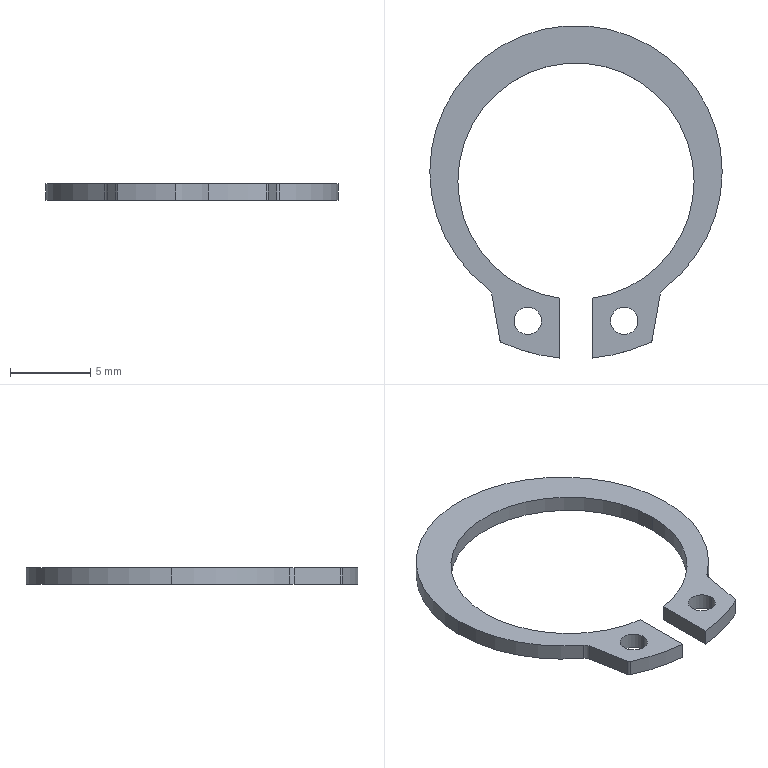Part | SolidWorks | features MoveCopyBody 1, Stock 1 | 1 solid | 22 faces | box 18.2 x 20.685 x 1 mm | volume 104.691 mm3 | cylinder 16 | plane 6 | commonest cylinder face diameters 1.7 x4 14.7 x3 18.2 x3 0.4 x2 1 x2 22.1 x2
STEP:
#1=CARTESIAN_POINT('',(2.15,-8.697,0.));
#2=VERTEX_POINT('',#1);
#3=CARTESIAN_POINT('',(3.85,-8.697,0.));
#4=VERTEX_POINT('',#3);
#5=CARTESIAN_POINT('',(3.,-8.697,0.));
#6=DIRECTION('',(0.,0.,1.));
#7=DIRECTION('',(-1.,0.,0.));
#8=AXIS2_PLACEMENT_3D('',#5,#6,#7);
#9=CIRCLE('',#8,0.85);
#10=EDGE_CURVE('',#2,#4,#9,.T.);
#11=ORIENTED_EDGE('',*,*,#10,.F.);
#12=CARTESIAN_POINT('',(2.15,-8.697,1.));
#13=VERTEX_POINT('',#12);
#14=CARTESIAN_POINT('',(2.15,-8.697,0.));
#15=DIRECTION('',(0.,0.,1.));
#16=VECTOR('',#15,1000.);
#17=LINE('',#14,#16);
#18=EDGE_CURVE('',#2,#13,#17,.T.);
#19=ORIENTED_EDGE('',*,*,#18,.T.);
#20=CARTESIAN_POINT('',(3.85,-8.697,1.));
#21=VERTEX_POINT('',#20);
#22=CARTESIAN_POINT('',(3.,-8.697,1.));
#23=DIRECTION('',(0.,0.,1.));
#24=DIRECTION('',(-1.,0.,0.));
#25=AXIS2_PLACEMENT_3D('',#22,#23,#24);
#26=CIRCLE('',#25,0.85);
#27=EDGE_CURVE('',#13,#21,#26,.T.);
#28=ORIENTED_EDGE('',*,*,#27,.T.);
#29=CARTESIAN_POINT('',(3.85,-8.697,0.));
#30=DIRECTION('',(0.,0.,1.));
#31=VECTOR('',#30,1000.);
#32=LINE('',#29,#31);
#33=EDGE_CURVE('',#4,#21,#32,.T.);
#34=ORIENTED_EDGE('',*,*,#33,.F.);
#35=EDGE_LOOP('',(#11,#19,#28,#34));
#36=FACE_OUTER_BOUND('',#35,.T.);
#37=CARTESIAN_POINT('',(3.,-8.697,0.));
#38=DIRECTION('',(0.,0.,1.));
#39=DIRECTION('',(1.,0.,0.));
#40=AXIS2_PLACEMENT_3D('',#37,#38,#39);
#41=CYLINDRICAL_SURFACE('',#40,0.85);
#42=ADVANCED_FACE('',(#36),#41,.F.);
#43=CARTESIAN_POINT('',(-3.85,-8.697,0.));
#44=VERTEX_POINT('',#43);
#45=CARTESIAN_POINT('',(-2.15,-8.697,0.));
#46=VERTEX_POINT('',#45);
#47=CARTESIAN_POINT('',(-3.,-8.697,0.));
#48=DIRECTION('',(0.,0.,1.));
#49=DIRECTION('',(1.,0.,0.));
#50=AXIS2_PLACEMENT_3D('',#47,#48,#49);
#51=CIRCLE('',#50,0.85);
#52=EDGE_CURVE('',#44,#46,#51,.T.);
#53=ORIENTED_EDGE('',*,*,#52,.F.);
#54=CARTESIAN_POINT('',(-3.85,-8.697,1.));
#55=VERTEX_POINT('',#54);
#56=CARTESIAN_POINT('',(-3.85,-8.697,0.));
#57=DIRECTION('',(0.,0.,1.));
#58=VECTOR('',#57,1000.);
#59=LINE('',#56,#58);
#60=EDGE_CURVE('',#44,#55,#59,.T.);
#61=ORIENTED_EDGE('',*,*,#60,.T.);
#62=CARTESIAN_POINT('',(-2.15,-8.697,1.));
#63=VERTEX_POINT('',#62);
#64=CARTESIAN_POINT('',(-3.,-8.697,1.));
#65=DIRECTION('',(0.,0.,1.));
#66=DIRECTION('',(1.,0.,0.));
#67=AXIS2_PLACEMENT_3D('',#64,#65,#66);
#68=CIRCLE('',#67,0.85);
#69=EDGE_CURVE('',#55,#63,#68,.T.);
#70=ORIENTED_EDGE('',*,*,#69,.T.);
#71=CARTESIAN_POINT('',(-2.15,-8.697,0.));
#72=DIRECTION('',(0.,0.,1.));
#73=VECTOR('',#72,1000.);
#74=LINE('',#71,#73);
#75=EDGE_CURVE('',#46,#63,#74,.T.);
#76=ORIENTED_EDGE('',*,*,#75,.F.);
#77=EDGE_LOOP('',(#53,#61,#70,#76));
#78=FACE_OUTER_BOUND('',#77,.T.);
#79=CARTESIAN_POINT('',(-3.,-8.697,0.));
#80=DIRECTION('',(0.,0.,1.));
#81=DIRECTION('',(1.,0.,0.));
#82=AXIS2_PLACEMENT_3D('',#79,#80,#81);
#83=CYLINDRICAL_SURFACE('',#82,0.85);
#84=ADVANCED_FACE('',(#78),#83,.F.);
#85=CARTESIAN_POINT('',(9.1,0.58,0.));
#86=VERTEX_POINT('',#85);
#87=CARTESIAN_POINT('',(-9.1,0.58,0.));
#88=VERTEX_POINT('',#87);
#89=CARTESIAN_POINT('',(0.,0.58,0.));
#90=DIRECTION('',(0.,0.,1.));
#91=DIRECTION('',(1.,0.,0.));
#92=AXIS2_PLACEMENT_3D('',#89,#90,#91);
#93=CIRCLE('',#92,9.1);
#94=EDGE_CURVE('',#86,#88,#93,.T.);
#95=ORIENTED_EDGE('',*,*,#94,.T.);
#96=CARTESIAN_POINT('',(-9.1,0.58,1.));
#97=VERTEX_POINT('',#96);
#98=CARTESIAN_POINT('',(-9.1,0.58,0.));
#99=DIRECTION('',(0.,0.,1.));
#100=VECTOR('',#99,1000.);
#101=LINE('',#98,#100);
#102=EDGE_CURVE('',#88,#97,#101,.T.);
#103=ORIENTED_EDGE('',*,*,#102,.T.);
#104=CARTESIAN_POINT('',(9.1,0.58,1.));
#105=VERTEX_POINT('',#104);
#106=CARTESIAN_POINT('',(0.,0.58,1.));
#107=DIRECTION('',(0.,0.,1.));
#108=DIRECTION('',(1.,0.,0.));
#109=AXIS2_PLACEMENT_3D('',#106,#107,#108);
#110=CIRCLE('',#109,9.1);
#111=EDGE_CURVE('',#105,#97,#110,.T.);
#112=ORIENTED_EDGE('',*,*,#111,.F.);
#113=CARTESIAN_POINT('',(9.1,0.58,0.));
#114=DIRECTION('',(0.,0.,1.));
#115=VECTOR('',#114,1000.);
#116=LINE('',#113,#115);
#117=EDGE_CURVE('',#86,#105,#116,.T.);
#118=ORIENTED_EDGE('',*,*,#117,.F.);
#119=EDGE_LOOP('',(#95,#103,#112,#118));
#120=FACE_OUTER_BOUND('',#119,.T.);
#121=CARTESIAN_POINT('',(0.,0.58,0.));
#122=DIRECTION('',(0.,0.,1.));
#123=DIRECTION('',(1.,0.,0.));
#124=AXIS2_PLACEMENT_3D('',#121,#122,#123);
#125=CYLINDRICAL_SURFACE('',#124,9.1);
#126=ADVANCED_FACE('',(#120),#125,.T.);
#127=CARTESIAN_POINT('',(5.437,-6.717,0.));
#128=VERTEX_POINT('',#127);
#129=CARTESIAN_POINT('',(0.,0.58,0.));
#130=DIRECTION('',(0.,0.,1.));
#131=DIRECTION('',(1.,0.,0.));
#132=AXIS2_PLACEMENT_3D('',#129,#130,#131);
#133=CIRCLE('',#132,9.1);
#134=EDGE_CURVE('',#128,#86,#133,.T.);
#135=ORIENTED_EDGE('',*,*,#134,.T.);
#136=ORIENTED_EDGE('',*,*,#117,.T.);
#137=CARTESIAN_POINT('',(5.437,-6.717,1.));
#138=VERTEX_POINT('',#137);
#139=CARTESIAN_POINT('',(0.,0.58,1.));
#140=DIRECTION('',(0.,0.,1.));
#141=DIRECTION('',(1.,0.,0.));
#142=AXIS2_PLACEMENT_3D('',#139,#140,#141);
#143=CIRCLE('',#142,9.1);
#144=EDGE_CURVE('',#138,#105,#143,.T.);
#145=ORIENTED_EDGE('',*,*,#144,.F.);
#146=CARTESIAN_POINT('',(5.437,-6.717,0.));
#147=DIRECTION('',(0.,0.,-1.));
#148=VECTOR('',#147,1000.);
#149=LINE('',#146,#148);
#150=EDGE_CURVE('',#138,#128,#149,.T.);
#151=ORIENTED_EDGE('',*,*,#150,.T.);
#152=EDGE_LOOP('',(#135,#136,#145,#151));
#153=FACE_OUTER_BOUND('',#152,.T.);
#154=CARTESIAN_POINT('',(0.,0.58,0.));
#155=DIRECTION('',(0.,0.,1.));
#156=DIRECTION('',(1.,0.,0.));
#157=AXIS2_PLACEMENT_3D('',#154,#155,#156);
#158=CYLINDRICAL_SURFACE('',#157,9.1);
#159=ADVANCED_FACE('',(#153),#158,.T.);
#160=CARTESIAN_POINT('',(-1.,-7.282,0.));
#161=VERTEX_POINT('',#160);
#162=CARTESIAN_POINT('',(-7.35,0.,0.));
#163=VERTEX_POINT('',#162);
#164=CARTESIAN_POINT('',(0.,0.,0.));
#165=DIRECTION('',(0.,0.,-1.));
#166=DIRECTION('',(1.,0.,0.));
#167=AXIS2_PLACEMENT_3D('',#164,#165,#166);
#168=CIRCLE('',#167,7.35);
#169=EDGE_CURVE('',#161,#163,#168,.T.);
#170=ORIENTED_EDGE('',*,*,#169,.T.);
#171=CARTESIAN_POINT('',(-7.35,0.,1.));
#172=VERTEX_POINT('',#171);
#173=CARTESIAN_POINT('',(-7.35,0.,0.));
#174=DIRECTION('',(0.,0.,1.));
#175=VECTOR('',#174,1000.);
#176=LINE('',#173,#175);
#177=EDGE_CURVE('',#163,#172,#176,.T.);
#178=ORIENTED_EDGE('',*,*,#177,.T.);
#179=CARTESIAN_POINT('',(-1.,-7.282,1.));
#180=VERTEX_POINT('',#179);
#181=CARTESIAN_POINT('',(0.,0.,1.));
#182=DIRECTION('',(0.,0.,-1.));
#183=DIRECTION('',(1.,0.,0.));
#184=AXIS2_PLACEMENT_3D('',#181,#182,#183);
#185=CIRCLE('',#184,7.35);
#186=EDGE_CURVE('',#180,#172,#185,.T.);
#187=ORIENTED_EDGE('',*,*,#186,.F.);
#188=CARTESIAN_POINT('',(-1.,-7.282,0.));
#189=DIRECTION('',(0.,0.,1.));
#190=VECTOR('',#189,1000.);
#191=LINE('',#188,#190);
#192=EDGE_CURVE('',#161,#180,#191,.T.);
#193=ORIENTED_EDGE('',*,*,#192,.F.);
#194=EDGE_LOOP('',(#170,#178,#187,#193));
#195=FACE_OUTER_BOUND('',#194,.T.);
#196=CARTESIAN_POINT('',(0.,0.,0.));
#197=DIRECTION('',(0.,0.,1.));
#198=DIRECTION('',(1.,0.,0.));
#199=AXIS2_PLACEMENT_3D('',#196,#197,#198);
#200=CYLINDRICAL_SURFACE('',#199,7.35);
#201=ADVANCED_FACE('',(#195),#200,.F.);
#202=ORIENTED_EDGE('',*,*,#177,.F.);
#203=CARTESIAN_POINT('',(7.35,0.,0.));
#204=VERTEX_POINT('',#203);
#205=CARTESIAN_POINT('',(0.,0.,0.));
#206=DIRECTION('',(0.,0.,-1.));
#207=DIRECTION('',(1.,0.,0.));
#208=AXIS2_PLACEMENT_3D('',#205,#206,#207);
#209=CIRCLE('',#208,7.35);
#210=EDGE_CURVE('',#163,#204,#209,.T.);
#211=ORIENTED_EDGE('',*,*,#210,.T.);
#212=CARTESIAN_POINT('',(7.35,0.,1.));
#213=VERTEX_POINT('',#212);
#214=CARTESIAN_POINT('',(7.35,0.,0.));
#215=DIRECTION('',(0.,0.,1.));
#216=VECTOR('',#215,1000.);
#217=LINE('',#214,#216);
#218=EDGE_CURVE('',#204,#213,#217,.T.);
#219=ORIENTED_EDGE('',*,*,#218,.T.);
#220=CARTESIAN_POINT('',(0.,0.,1.));
#221=DIRECTION('',(0.,0.,-1.));
#222=DIRECTION('',(1.,0.,0.));
#223=AXIS2_PLACEMENT_3D('',#220,#221,#222);
#224=CIRCLE('',#223,7.35);
#225=EDGE_CURVE('',#172,#213,#224,.T.);
#226=ORIENTED_EDGE('',*,*,#225,.F.);
#227=EDGE_LOOP('',(#202,#211,#219,#226));
#228=FACE_OUTER_BOUND('',#227,.T.);
#229=CARTESIAN_POINT('',(0.,0.,0.));
#230=DIRECTION('',(0.,0.,1.));
#231=DIRECTION('',(1.,0.,0.));
#232=AXIS2_PLACEMENT_3D('',#229,#230,#231);
#233=CYLINDRICAL_SURFACE('',#232,7.35);
#234=ADVANCED_FACE('',(#228),#233,.F.);
#235=CARTESIAN_POINT('',(1.,-11.005,0.));
#236=VERTEX_POINT('',#235);
#237=CARTESIAN_POINT('',(4.626,-10.035,0.));
#238=VERTEX_POINT('',#237);
#239=CARTESIAN_POINT('',(0.,0.,0.));
#240=DIRECTION('',(0.,0.,1.));
#241=DIRECTION('',(-1.,0.,0.));
#242=AXIS2_PLACEMENT_3D('',#239,#240,#241);
#243=CIRCLE('',#242,11.05);
#244=EDGE_CURVE('',#236,#238,#243,.T.);
#245=ORIENTED_EDGE('',*,*,#244,.T.);
#246=CARTESIAN_POINT('',(4.626,-10.035,1.));
#247=VERTEX_POINT('',#246);
#248=CARTESIAN_POINT('',(4.626,-10.035,0.));
#249=DIRECTION('',(0.,0.,1.));
#250=VECTOR('',#249,1000.);
#251=LINE('',#248,#250);
#252=EDGE_CURVE('',#238,#247,#251,.T.);
#253=ORIENTED_EDGE('',*,*,#252,.T.);
#254=CARTESIAN_POINT('',(1.,-11.005,1.));
#255=VERTEX_POINT('',#254);
#256=CARTESIAN_POINT('',(0.,0.,1.));
#257=DIRECTION('',(0.,0.,1.));
#258=DIRECTION('',(-1.,0.,0.));
#259=AXIS2_PLACEMENT_3D('',#256,#257,#258);
#260=CIRCLE('',#259,11.05);
#261=EDGE_CURVE('',#255,#247,#260,.T.);
#262=ORIENTED_EDGE('',*,*,#261,.F.);
#263=CARTESIAN_POINT('',(1.,-11.005,0.));
#264=DIRECTION('',(0.,0.,1.));
#265=VECTOR('',#264,1000.);
#266=LINE('',#263,#265);
#267=EDGE_CURVE('',#236,#255,#266,.T.);
#268=ORIENTED_EDGE('',*,*,#267,.F.);
#269=EDGE_LOOP('',(#245,#253,#262,#268));
#270=FACE_OUTER_BOUND('',#269,.T.);
#271=CARTESIAN_POINT('',(0.,0.,0.));
#272=DIRECTION('',(0.,0.,1.));
#273=DIRECTION('',(1.,0.,0.));
#274=AXIS2_PLACEMENT_3D('',#271,#272,#273);
#275=CYLINDRICAL_SURFACE('',#274,11.05);
#276=ADVANCED_FACE('',(#270),#275,.T.);
#277=CARTESIAN_POINT('',(1.,-7.282,1.));
#278=VERTEX_POINT('',#277);
#279=CARTESIAN_POINT('',(1.,-7.282,1.));
#280=DIRECTION('',(0.,-1.,0.));
#281=VECTOR('',#280,1000.);
#282=LINE('',#279,#281);
#283=EDGE_CURVE('',#278,#255,#282,.T.);
#284=ORIENTED_EDGE('',*,*,#283,.F.);
#285=CARTESIAN_POINT('',(1.,-7.282,0.));
#286=VERTEX_POINT('',#285);
#287=CARTESIAN_POINT('',(1.,-7.282,0.));
#288=DIRECTION('',(0.,0.,1.));
#289=VECTOR('',#288,1000.);
#290=LINE('',#287,#289);
#291=EDGE_CURVE('',#286,#278,#290,.T.);
#292=ORIENTED_EDGE('',*,*,#291,.F.);
#293=CARTESIAN_POINT('',(1.,-7.282,0.));
#294=DIRECTION('',(0.,-1.,0.));
#295=VECTOR('',#294,1000.);
#296=LINE('',#293,#295);
#297=EDGE_CURVE('',#286,#236,#296,.T.);
#298=ORIENTED_EDGE('',*,*,#297,.T.);
#299=ORIENTED_EDGE('',*,*,#267,.T.);
#300=EDGE_LOOP('',(#284,#292,#298,#299));
#301=FACE_OUTER_BOUND('',#300,.T.);
#302=CARTESIAN_POINT('',(1.,-7.282,0.));
#303=DIRECTION('',(-1.,0.,0.));
#304=DIRECTION('',(0.,0.,1.));
#305=AXIS2_PLACEMENT_3D('',#302,#303,#304);
#306=PLANE('',#305);
#307=ADVANCED_FACE('',(#301),#306,.T.);
#308=ORIENTED_EDGE('',*,*,#218,.F.);
#309=CARTESIAN_POINT('',(0.,0.,0.));
#310=DIRECTION('',(0.,0.,-1.));
#311=DIRECTION('',(1.,0.,0.));
#312=AXIS2_PLACEMENT_3D('',#309,#310,#311);
#313=CIRCLE('',#312,7.35);
#314=EDGE_CURVE('',#204,#286,#313,.T.);
#315=ORIENTED_EDGE('',*,*,#314,.T.);
#316=ORIENTED_EDGE('',*,*,#291,.T.);
#317=CARTESIAN_POINT('',(0.,0.,1.));
#318=DIRECTION('',(0.,0.,-1.));
#319=DIRECTION('',(1.,0.,0.));
#320=AXIS2_PLACEMENT_3D('',#317,#318,#319);
#321=CIRCLE('',#320,7.35);
#322=EDGE_CURVE('',#213,#278,#321,.T.);
#323=ORIENTED_EDGE('',*,*,#322,.F.);
#324=EDGE_LOOP('',(#308,#315,#316,#323));
#325=FACE_OUTER_BOUND('',#324,.T.);
#326=CARTESIAN_POINT('',(0.,0.,0.));
#327=DIRECTION('',(0.,0.,1.));
#328=DIRECTION('',(1.,0.,0.));
#329=AXIS2_PLACEMENT_3D('',#326,#327,#328);
#330=CYLINDRICAL_SURFACE('',#329,7.35);
#331=ADVANCED_FACE('',(#325),#330,.F.);
#332=CARTESIAN_POINT('',(-1.,-11.005,1.));
#333=VERTEX_POINT('',#332);
#334=CARTESIAN_POINT('',(-1.,-7.282,1.));
#335=DIRECTION('',(0.,1.,0.));
#336=VECTOR('',#335,1000.);
#337=LINE('',#334,#336);
#338=EDGE_CURVE('',#333,#180,#337,.T.);
#339=ORIENTED_EDGE('',*,*,#338,.F.);
#340=CARTESIAN_POINT('',(-1.,-11.005,0.));
#341=VERTEX_POINT('',#340);
#342=CARTESIAN_POINT('',(-1.,-11.005,0.));
#343=DIRECTION('',(0.,0.,1.));
#344=VECTOR('',#343,1000.);
#345=LINE('',#342,#344);
#346=EDGE_CURVE('',#341,#333,#345,.T.);
#347=ORIENTED_EDGE('',*,*,#346,.F.);
#348=CARTESIAN_POINT('',(-1.,-7.282,0.));
#349=DIRECTION('',(0.,1.,0.));
#350=VECTOR('',#349,1000.);
#351=LINE('',#348,#350);
#352=EDGE_CURVE('',#341,#161,#351,.T.);
#353=ORIENTED_EDGE('',*,*,#352,.T.);
#354=ORIENTED_EDGE('',*,*,#192,.T.);
#355=EDGE_LOOP('',(#339,#347,#353,#354));
#356=FACE_OUTER_BOUND('',#355,.T.);
#357=CARTESIAN_POINT('',(-1.,-7.282,0.));
#358=DIRECTION('',(1.,0.,0.));
#359=DIRECTION('',(0.,0.,-1.));
#360=AXIS2_PLACEMENT_3D('',#357,#358,#359);
#361=PLANE('',#360);
#362=ADVANCED_FACE('',(#356),#361,.T.);
#363=CARTESIAN_POINT('',(-4.626,-10.035,1.));
#364=VERTEX_POINT('',#363);
#365=CARTESIAN_POINT('',(0.,0.,1.));
#366=DIRECTION('',(0.,0.,1.));
#367=DIRECTION('',(1.,0.,0.));
#368=AXIS2_PLACEMENT_3D('',#365,#366,#367);
#369=CIRCLE('',#368,11.05);
#370=EDGE_CURVE('',#364,#333,#369,.T.);
#371=ORIENTED_EDGE('',*,*,#370,.F.);
#372=CARTESIAN_POINT('',(-4.626,-10.035,0.));
#373=VERTEX_POINT('',#372);
#374=CARTESIAN_POINT('',(-4.626,-10.035,0.));
#375=DIRECTION('',(0.,0.,-1.));
#376=VECTOR('',#375,1000.);
#377=LINE('',#374,#376);
#378=EDGE_CURVE('',#364,#373,#377,.T.);
#379=ORIENTED_EDGE('',*,*,#378,.T.);
#380=CARTESIAN_POINT('',(0.,0.,0.));
#381=DIRECTION('',(0.,0.,1.));
#382=DIRECTION('',(1.,0.,0.));
#383=AXIS2_PLACEMENT_3D('',#380,#381,#382);
#384=CIRCLE('',#383,11.05);
#385=EDGE_CURVE('',#373,#341,#384,.T.);
#386=ORIENTED_EDGE('',*,*,#385,.T.);
#387=ORIENTED_EDGE('',*,*,#346,.T.);
#388=EDGE_LOOP('',(#371,#379,#386,#387));
#389=FACE_OUTER_BOUND('',#388,.T.);
#390=CARTESIAN_POINT('',(0.,0.,0.));
#391=DIRECTION('',(0.,0.,1.));
#392=DIRECTION('',(1.,0.,0.));
#393=AXIS2_PLACEMENT_3D('',#390,#391,#392);
#394=CYLINDRICAL_SURFACE('',#393,11.05);
#395=ADVANCED_FACE('',(#389),#394,.T.);
#396=CARTESIAN_POINT('',(-5.243,-7.031,1.));
#397=VERTEX_POINT('',#396);
#398=CARTESIAN_POINT('',(-4.74,-9.888,1.));
#399=VERTEX_POINT('',#398);
#400=CARTESIAN_POINT('',(-5.278,-6.833,1.));
#401=DIRECTION('',(0.1736,-0.9848,0.));
#402=VECTOR('',#401,1000.);
#403=LINE('',#400,#402);
#404=EDGE_CURVE('',#397,#399,#403,.T.);
#405=ORIENTED_EDGE('',*,*,#404,.F.);
#406=CARTESIAN_POINT('',(-5.243,-7.031,0.));
#407=VERTEX_POINT('',#406);
#408=CARTESIAN_POINT('',(-5.243,-7.031,0.));
#409=DIRECTION('',(0.,0.,-1.));
#410=VECTOR('',#409,1000.);
#411=LINE('',#408,#410);
#412=EDGE_CURVE('',#397,#407,#411,.T.);
#413=ORIENTED_EDGE('',*,*,#412,.T.);
#414=CARTESIAN_POINT('',(-4.74,-9.888,0.));
#415=VERTEX_POINT('',#414);
#416=CARTESIAN_POINT('',(-5.278,-6.833,0.));
#417=DIRECTION('',(0.1736,-0.9848,0.));
#418=VECTOR('',#417,1000.);
#419=LINE('',#416,#418);
#420=EDGE_CURVE('',#407,#415,#419,.T.);
#421=ORIENTED_EDGE('',*,*,#420,.T.);
#422=CARTESIAN_POINT('',(-4.74,-9.888,0.));
#423=DIRECTION('',(0.,0.,1.));
#424=VECTOR('',#423,1000.);
#425=LINE('',#422,#424);
#426=EDGE_CURVE('',#415,#399,#425,.T.);
#427=ORIENTED_EDGE('',*,*,#426,.T.);
#428=EDGE_LOOP('',(#405,#413,#421,#427));
#429=FACE_OUTER_BOUND('',#428,.T.);
#430=CARTESIAN_POINT('',(-5.278,-6.833,0.));
#431=DIRECTION('',(-0.9848,-0.1736,0.));
#432=DIRECTION('',(0.1736,-0.9848,0.));
#433=AXIS2_PLACEMENT_3D('',#430,#431,#432);
#434=PLANE('',#433);
#435=ADVANCED_FACE('',(#429),#434,.T.);
#436=ORIENTED_EDGE('',*,*,#102,.F.);
#437=CARTESIAN_POINT('',(-5.437,-6.717,0.));
#438=VERTEX_POINT('',#437);
#439=CARTESIAN_POINT('',(0.,0.58,0.));
#440=DIRECTION('',(0.,0.,1.));
#441=DIRECTION('',(1.,0.,0.));
#442=AXIS2_PLACEMENT_3D('',#439,#440,#441);
#443=CIRCLE('',#442,9.1);
#444=EDGE_CURVE('',#88,#438,#443,.T.);
#445=ORIENTED_EDGE('',*,*,#444,.T.);
#446=CARTESIAN_POINT('',(-5.437,-6.717,1.));
#447=VERTEX_POINT('',#446);
#448=CARTESIAN_POINT('',(-5.437,-6.717,0.));
#449=DIRECTION('',(0.,0.,1.));
#450=VECTOR('',#449,1000.);
#451=LINE('',#448,#450);
#452=EDGE_CURVE('',#438,#447,#451,.T.);
#453=ORIENTED_EDGE('',*,*,#452,.T.);
#454=CARTESIAN_POINT('',(0.,0.58,1.));
#455=DIRECTION('',(0.,0.,1.));
#456=DIRECTION('',(1.,0.,0.));
#457=AXIS2_PLACEMENT_3D('',#454,#455,#456);
#458=CIRCLE('',#457,9.1);
#459=EDGE_CURVE('',#97,#447,#458,.T.);
#460=ORIENTED_EDGE('',*,*,#459,.F.);
#461=EDGE_LOOP('',(#436,#445,#453,#460));
#462=FACE_OUTER_BOUND('',#461,.T.);
#463=CARTESIAN_POINT('',(0.,0.58,0.));
#464=DIRECTION('',(0.,0.,1.));
#465=DIRECTION('',(1.,0.,0.));
#466=AXIS2_PLACEMENT_3D('',#463,#464,#465);
#467=CYLINDRICAL_SURFACE('',#466,9.1);
#468=ADVANCED_FACE('',(#462),#467,.T.);
#469=CARTESIAN_POINT('',(4.74,-9.888,0.));
#470=VERTEX_POINT('',#469);
#471=CARTESIAN_POINT('',(5.243,-7.031,0.));
#472=VERTEX_POINT('',#471);
#473=CARTESIAN_POINT('',(5.278,-6.833,0.));
#474=DIRECTION('',(0.1736,0.9848,0.));
#475=VECTOR('',#474,1000.);
#476=LINE('',#473,#475);
#477=EDGE_CURVE('',#470,#472,#476,.T.);
#478=ORIENTED_EDGE('',*,*,#477,.T.);
#479=CARTESIAN_POINT('',(5.243,-7.031,1.));
#480=VERTEX_POINT('',#479);
#481=CARTESIAN_POINT('',(5.243,-7.031,1.));
#482=DIRECTION('',(0.,0.,1.));
#483=VECTOR('',#482,1000.);
#484=LINE('',#481,#483);
#485=EDGE_CURVE('',#472,#480,#484,.T.);
#486=ORIENTED_EDGE('',*,*,#485,.T.);
#487=CARTESIAN_POINT('',(4.74,-9.888,1.));
#488=VERTEX_POINT('',#487);
#489=CARTESIAN_POINT('',(5.278,-6.833,1.));
#490=DIRECTION('',(0.1736,0.9848,0.));
#491=VECTOR('',#490,1000.);
#492=LINE('',#489,#491);
#493=EDGE_CURVE('',#488,#480,#492,.T.);
#494=ORIENTED_EDGE('',*,*,#493,.F.);
#495=CARTESIAN_POINT('',(4.74,-9.888,0.));
#496=DIRECTION('',(0.,0.,-1.));
#497=VECTOR('',#496,1000.);
#498=LINE('',#495,#497);
#499=EDGE_CURVE('',#488,#470,#498,.T.);
#500=ORIENTED_EDGE('',*,*,#499,.T.);
#501=EDGE_LOOP('',(#478,#486,#494,#500));
#502=FACE_OUTER_BOUND('',#501,.T.);
#503=CARTESIAN_POINT('',(5.278,-6.833,0.));
#504=DIRECTION('',(0.9848,-0.1736,0.));
#505=DIRECTION('',(0.1736,0.9848,0.));
#506=AXIS2_PLACEMENT_3D('',#503,#504,#505);
#507=PLANE('',#506);
#508=ADVANCED_FACE('',(#502),#507,.T.);
#509=CARTESIAN_POINT('',(3.,-8.697,0.));
#510=DIRECTION('',(0.,0.,1.));
#511=DIRECTION('',(-1.,0.,0.));
#512=AXIS2_PLACEMENT_3D('',#509,#510,#511);
#513=CIRCLE('',#512,0.85);
#514=EDGE_CURVE('',#4,#2,#513,.T.);
#515=ORIENTED_EDGE('',*,*,#514,.T.);
#516=ORIENTED_EDGE('',*,*,#10,.T.);
#517=EDGE_LOOP('',(#515,#516));
#518=FACE_BOUND('',#517,.T.);
#519=CARTESIAN_POINT('',(-3.,-8.697,0.));
#520=DIRECTION('',(0.,0.,1.));
#521=DIRECTION('',(1.,0.,0.));
#522=AXIS2_PLACEMENT_3D('',#519,#520,#521);
#523=CIRCLE('',#522,0.85);
#524=EDGE_CURVE('',#46,#44,#523,.T.);
#525=ORIENTED_EDGE('',*,*,#524,.T.);
#526=ORIENTED_EDGE('',*,*,#52,.T.);
#527=EDGE_LOOP('',(#525,#526));
#528=FACE_BOUND('',#527,.T.);
#529=ORIENTED_EDGE('',*,*,#385,.F.);
#530=CARTESIAN_POINT('',(-4.543,-9.853,0.));
#531=DIRECTION('',(0.,0.,-1.));
#532=DIRECTION('',(-1.,0.,0.));
#533=AXIS2_PLACEMENT_3D('',#530,#531,#532);
#534=CIRCLE('',#533,0.2);
#535=EDGE_CURVE('',#373,#415,#534,.T.);
#536=ORIENTED_EDGE('',*,*,#535,.T.);
#537=ORIENTED_EDGE('',*,*,#420,.F.);
#538=CARTESIAN_POINT('',(-5.736,-7.118,0.));
#539=DIRECTION('',(0.,0.,1.));
#540=DIRECTION('',(-1.,0.,0.));
#541=AXIS2_PLACEMENT_3D('',#538,#539,#540);
#542=CIRCLE('',#541,0.5);
#543=EDGE_CURVE('',#407,#438,#542,.T.);
#544=ORIENTED_EDGE('',*,*,#543,.T.);
#545=ORIENTED_EDGE('',*,*,#444,.F.);
#546=ORIENTED_EDGE('',*,*,#94,.F.);
#547=ORIENTED_EDGE('',*,*,#134,.F.);
#548=CARTESIAN_POINT('',(5.736,-7.118,0.));
#549=DIRECTION('',(0.,0.,1.));
#550=DIRECTION('',(-1.,0.,0.));
#551=AXIS2_PLACEMENT_3D('',#548,#549,#550);
#552=CIRCLE('',#551,0.5);
#553=EDGE_CURVE('',#128,#472,#552,.T.);
#554=ORIENTED_EDGE('',*,*,#553,.T.);
#555=ORIENTED_EDGE('',*,*,#477,.F.);
#556=CARTESIAN_POINT('',(4.543,-9.853,0.));
#557=DIRECTION('',(0.,0.,-1.));
#558=DIRECTION('',(-1.,0.,0.));
#559=AXIS2_PLACEMENT_3D('',#556,#557,#558);
#560=CIRCLE('',#559,0.2);
#561=EDGE_CURVE('',#470,#238,#560,.T.);
#562=ORIENTED_EDGE('',*,*,#561,.T.);
#563=ORIENTED_EDGE('',*,*,#244,.F.);
#564=ORIENTED_EDGE('',*,*,#297,.F.);
#565=ORIENTED_EDGE('',*,*,#314,.F.);
#566=ORIENTED_EDGE('',*,*,#210,.F.);
#567=ORIENTED_EDGE('',*,*,#169,.F.);
#568=ORIENTED_EDGE('',*,*,#352,.F.);
#569=EDGE_LOOP('',(#529,#536,#537,#544,#545,#546,#547,#554,#555,#562,#563,#564,#565,#566,#567,#568));
#570=FACE_OUTER_BOUND('',#569,.T.);
#571=CARTESIAN_POINT('',(0.,0.,0.));
#572=DIRECTION('',(0.,0.,-1.));
#573=DIRECTION('',(-1.,0.,0.));
#574=AXIS2_PLACEMENT_3D('',#571,#572,#573);
#575=PLANE('',#574);
#576=ADVANCED_FACE('',(#518,#528,#570),#575,.T.);
#577=CARTESIAN_POINT('',(3.,-8.697,1.));
#578=DIRECTION('',(0.,0.,1.));
#579=DIRECTION('',(-1.,0.,0.));
#580=AXIS2_PLACEMENT_3D('',#577,#578,#579);
#581=CIRCLE('',#580,0.85);
#582=EDGE_CURVE('',#21,#13,#581,.T.);
#583=ORIENTED_EDGE('',*,*,#582,.F.);
#584=ORIENTED_EDGE('',*,*,#27,.F.);
#585=EDGE_LOOP('',(#583,#584));
#586=FACE_BOUND('',#585,.T.);
#587=CARTESIAN_POINT('',(-3.,-8.697,1.));
#588=DIRECTION('',(0.,0.,1.));
#589=DIRECTION('',(1.,0.,0.));
#590=AXIS2_PLACEMENT_3D('',#587,#588,#589);
#591=CIRCLE('',#590,0.85);
#592=EDGE_CURVE('',#63,#55,#591,.T.);
#593=ORIENTED_EDGE('',*,*,#592,.F.);
#594=ORIENTED_EDGE('',*,*,#69,.F.);
#595=EDGE_LOOP('',(#593,#594));
#596=FACE_BOUND('',#595,.T.);
#597=ORIENTED_EDGE('',*,*,#144,.T.);
#598=ORIENTED_EDGE('',*,*,#111,.T.);
#599=ORIENTED_EDGE('',*,*,#459,.T.);
#600=CARTESIAN_POINT('',(-5.736,-7.118,1.));
#601=DIRECTION('',(0.,0.,-1.));
#602=DIRECTION('',(-1.,0.,0.));
#603=AXIS2_PLACEMENT_3D('',#600,#601,#602);
#604=CIRCLE('',#603,0.5);
#605=EDGE_CURVE('',#447,#397,#604,.T.);
#606=ORIENTED_EDGE('',*,*,#605,.T.);
#607=ORIENTED_EDGE('',*,*,#404,.T.);
#608=CARTESIAN_POINT('',(-4.543,-9.853,1.));
#609=DIRECTION('',(0.,0.,1.));
#610=DIRECTION('',(-1.,0.,0.));
#611=AXIS2_PLACEMENT_3D('',#608,#609,#610);
#612=CIRCLE('',#611,0.2);
#613=EDGE_CURVE('',#399,#364,#612,.T.);
#614=ORIENTED_EDGE('',*,*,#613,.T.);
#615=ORIENTED_EDGE('',*,*,#370,.T.);
#616=ORIENTED_EDGE('',*,*,#338,.T.);
#617=ORIENTED_EDGE('',*,*,#186,.T.);
#618=ORIENTED_EDGE('',*,*,#225,.T.);
#619=ORIENTED_EDGE('',*,*,#322,.T.);
#620=ORIENTED_EDGE('',*,*,#283,.T.);
#621=ORIENTED_EDGE('',*,*,#261,.T.);
#622=CARTESIAN_POINT('',(4.543,-9.853,1.));
#623=DIRECTION('',(0.,0.,1.));
#624=DIRECTION('',(-1.,0.,0.));
#625=AXIS2_PLACEMENT_3D('',#622,#623,#624);
#626=CIRCLE('',#625,0.2);
#627=EDGE_CURVE('',#247,#488,#626,.T.);
#628=ORIENTED_EDGE('',*,*,#627,.T.);
#629=ORIENTED_EDGE('',*,*,#493,.T.);
#630=CARTESIAN_POINT('',(5.736,-7.118,1.));
#631=DIRECTION('',(0.,0.,-1.));
#632=DIRECTION('',(-1.,0.,0.));
#633=AXIS2_PLACEMENT_3D('',#630,#631,#632);
#634=CIRCLE('',#633,0.5);
#635=EDGE_CURVE('',#480,#138,#634,.T.);
#636=ORIENTED_EDGE('',*,*,#635,.T.);
#637=EDGE_LOOP('',(#597,#598,#599,#606,#607,#614,#615,#616,#617,#618,#619,#620,#621,#628,#629,#636));
#638=FACE_OUTER_BOUND('',#637,.T.);
#639=CARTESIAN_POINT('',(0.,0.,1.));
#640=DIRECTION('',(0.,0.,-1.));
#641=DIRECTION('',(-1.,0.,0.));
#642=AXIS2_PLACEMENT_3D('',#639,#640,#641);
#643=PLANE('',#642);
#644=ADVANCED_FACE('',(#586,#596,#638),#643,.F.);
#645=ORIENTED_EDGE('',*,*,#60,.F.);
#646=ORIENTED_EDGE('',*,*,#524,.F.);
#647=ORIENTED_EDGE('',*,*,#75,.T.);
#648=ORIENTED_EDGE('',*,*,#592,.T.);
#649=EDGE_LOOP('',(#645,#646,#647,#648));
#650=FACE_OUTER_BOUND('',#649,.T.);
#651=CARTESIAN_POINT('',(-3.,-8.697,0.));
#652=DIRECTION('',(0.,0.,1.));
#653=DIRECTION('',(1.,0.,0.));
#654=AXIS2_PLACEMENT_3D('',#651,#652,#653);
#655=CYLINDRICAL_SURFACE('',#654,0.85);
#656=ADVANCED_FACE('',(#650),#655,.F.);
#657=ORIENTED_EDGE('',*,*,#18,.F.);
#658=ORIENTED_EDGE('',*,*,#514,.F.);
#659=ORIENTED_EDGE('',*,*,#33,.T.);
#660=ORIENTED_EDGE('',*,*,#582,.T.);
#661=EDGE_LOOP('',(#657,#658,#659,#660));
#662=FACE_OUTER_BOUND('',#661,.T.);
#663=CARTESIAN_POINT('',(3.,-8.697,0.));
#664=DIRECTION('',(0.,0.,1.));
#665=DIRECTION('',(1.,0.,0.));
#666=AXIS2_PLACEMENT_3D('',#663,#664,#665);
#667=CYLINDRICAL_SURFACE('',#666,0.85);
#668=ADVANCED_FACE('',(#662),#667,.F.);
#669=ORIENTED_EDGE('',*,*,#535,.F.);
#670=ORIENTED_EDGE('',*,*,#378,.F.);
#671=ORIENTED_EDGE('',*,*,#613,.F.);
#672=ORIENTED_EDGE('',*,*,#426,.F.);
#673=EDGE_LOOP('',(#669,#670,#671,#672));
#674=FACE_OUTER_BOUND('',#673,.T.);
#675=CARTESIAN_POINT('',(-4.543,-9.853,0.));
#676=DIRECTION('',(0.,0.,1.));
#677=DIRECTION('',(1.,0.,0.));
#678=AXIS2_PLACEMENT_3D('',#675,#676,#677);
#679=CYLINDRICAL_SURFACE('',#678,0.2);
#680=ADVANCED_FACE('',(#674),#679,.T.);
#681=ORIENTED_EDGE('',*,*,#561,.F.);
#682=ORIENTED_EDGE('',*,*,#499,.F.);
#683=ORIENTED_EDGE('',*,*,#627,.F.);
#684=ORIENTED_EDGE('',*,*,#252,.F.);
#685=EDGE_LOOP('',(#681,#682,#683,#684));
#686=FACE_OUTER_BOUND('',#685,.T.);
#687=CARTESIAN_POINT('',(4.543,-9.853,0.));
#688=DIRECTION('',(0.,0.,1.));
#689=DIRECTION('',(1.,0.,0.));
#690=AXIS2_PLACEMENT_3D('',#687,#688,#689);
#691=CYLINDRICAL_SURFACE('',#690,0.2);
#692=ADVANCED_FACE('',(#686),#691,.T.);
#693=ORIENTED_EDGE('',*,*,#553,.F.);
#694=ORIENTED_EDGE('',*,*,#150,.F.);
#695=ORIENTED_EDGE('',*,*,#635,.F.);
#696=ORIENTED_EDGE('',*,*,#485,.F.);
#697=EDGE_LOOP('',(#693,#694,#695,#696));
#698=FACE_OUTER_BOUND('',#697,.T.);
#699=CARTESIAN_POINT('',(5.736,-7.118,0.));
#700=DIRECTION('',(0.,0.,1.));
#701=DIRECTION('',(1.,0.,0.));
#702=AXIS2_PLACEMENT_3D('',#699,#700,#701);
#703=CYLINDRICAL_SURFACE('',#702,0.5);
#704=ADVANCED_FACE('',(#698),#703,.F.);
#705=ORIENTED_EDGE('',*,*,#543,.F.);
#706=ORIENTED_EDGE('',*,*,#412,.F.);
#707=ORIENTED_EDGE('',*,*,#605,.F.);
#708=ORIENTED_EDGE('',*,*,#452,.F.);
#709=EDGE_LOOP('',(#705,#706,#707,#708));
#710=FACE_OUTER_BOUND('',#709,.T.);
#711=CARTESIAN_POINT('',(-5.736,-7.118,0.));
#712=DIRECTION('',(0.,0.,1.));
#713=DIRECTION('',(1.,0.,0.));
#714=AXIS2_PLACEMENT_3D('',#711,#712,#713);
#715=CYLINDRICAL_SURFACE('',#714,0.5);
#716=ADVANCED_FACE('',(#710),#715,.F.);
#717=CLOSED_SHELL('',(#42,#84,#126,#159,#201,#234,#276,#307,#331,#362,#395,#435,#468,#508,#576,#644,#656,#668,#680,#692,#704,#716));
#718=MANIFOLD_SOLID_BREP('',#717);
#719=CARTESIAN_POINT('',(0.,0.,0.));
#720=DIRECTION('',(0.,0.,1.));
#721=DIRECTION('',(1.,0.,0.));
#722=AXIS2_PLACEMENT_3D('',#719,#720,#721);
#723=(LENGTH_UNIT()NAMED_UNIT(*)SI_UNIT(.MILLI.,.METRE.));
#724=UNCERTAINTY_MEASURE_WITH_UNIT(LENGTH_MEASURE(0.00001),#723,'','');
#725=(NAMED_UNIT(*)PLANE_ANGLE_UNIT()SI_UNIT($,.RADIAN.));
#726=(NAMED_UNIT(*)SI_UNIT($,.STERADIAN.)SOLID_ANGLE_UNIT());
#727=(GEOMETRIC_REPRESENTATION_CONTEXT(3)GLOBAL_UNCERTAINTY_ASSIGNED_CONTEXT((#724))GLOBAL_UNIT_ASSIGNED_CONTEXT((#723,#725,#726))REPRESENTATION_CONTEXT('',''));
#728=ADVANCED_BREP_SHAPE_REPRESENTATION('',(#718,#722),#727);